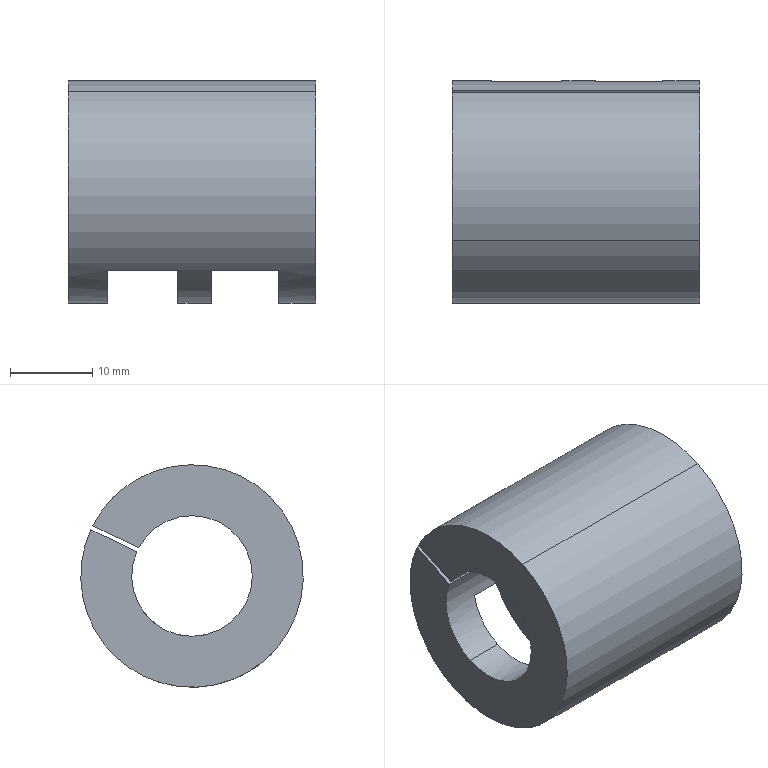Part | NX | 1 solid | 18 faces | box 30 x 27 x 27 mm | volume 9581 mm3 | plane 12 | cylinder 6 | commonest cylinder face diameters 14.64 x3 27 x3
STEP:
#1=CARTESIAN_POINT('',(15.301,-535.026,2413.504));
#2=VERTEX_POINT('',#1);
#3=CARTESIAN_POINT('',(15.301,-544.682,2416.678));
#4=VERTEX_POINT('',#3);
#5=CARTESIAN_POINT('',(15.301,-541.499,2410.086));
#6=DIRECTION('',(1.,0.,0.));
#7=DIRECTION('',(0.,-0.4348,0.9005));
#8=AXIS2_PLACEMENT_3D('',#5,#6,#7);
#9=CIRCLE('',#8,7.32);
#10=EDGE_CURVE('',#2,#4,#9,.T.);
#11=ORIENTED_EDGE('',*,*,#10,.T.);
#12=CARTESIAN_POINT('',(-14.699,-544.682,2416.678));
#13=VERTEX_POINT('',#12);
#14=CARTESIAN_POINT('',(15.301,-544.682,2416.678));
#15=DIRECTION('',(-1.,0.,0.));
#16=VECTOR('',#15,1.);
#17=LINE('',#14,#16);
#18=EDGE_CURVE('',#4,#13,#17,.T.);
#19=ORIENTED_EDGE('',*,*,#18,.T.);
#20=CARTESIAN_POINT('',(-14.699,-535.026,2413.504));
#21=VERTEX_POINT('',#20);
#22=CARTESIAN_POINT('',(-14.699,-541.499,2410.086));
#23=DIRECTION('',(1.,0.,0.));
#24=DIRECTION('',(0.,-0.4348,0.9005));
#25=AXIS2_PLACEMENT_3D('',#22,#23,#24);
#26=CIRCLE('',#25,7.32);
#27=EDGE_CURVE('',#21,#13,#26,.T.);
#28=ORIENTED_EDGE('',*,*,#27,.F.);
#29=CARTESIAN_POINT('',(15.301,-535.026,2413.504));
#30=DIRECTION('',(-1.,0.,0.));
#31=VECTOR('',#30,1.);
#32=LINE('',#29,#31);
#33=EDGE_CURVE('',#2,#21,#32,.T.);
#34=ORIENTED_EDGE('',*,*,#33,.F.);
#35=EDGE_LOOP('',(#11,#19,#28,#34));
#36=FACE_OUTER_BOUND('',#35,.T.);
#37=CARTESIAN_POINT('',(15.301,-541.499,2410.086));
#38=DIRECTION('',(-1.,0.,0.));
#39=DIRECTION('',(0.,0.4348,-0.9005));
#40=AXIS2_PLACEMENT_3D('',#37,#38,#39);
#41=CYLINDRICAL_SURFACE('',#40,7.32);
#42=ADVANCED_FACE('',(#36),#41,.F.);
#43=ORIENTED_EDGE('',*,*,#18,.F.);
#44=CARTESIAN_POINT('',(15.301,-538.317,2403.494));
#45=VERTEX_POINT('',#44);
#46=CARTESIAN_POINT('',(15.301,-541.499,2410.086));
#47=DIRECTION('',(1.,0.,0.));
#48=DIRECTION('',(0.,-0.4348,0.9005));
#49=AXIS2_PLACEMENT_3D('',#46,#47,#48);
#50=CIRCLE('',#49,7.32);
#51=EDGE_CURVE('',#4,#45,#50,.T.);
#52=ORIENTED_EDGE('',*,*,#51,.T.);
#53=CARTESIAN_POINT('',(10.819,-538.317,2403.494));
#54=VERTEX_POINT('',#53);
#55=CARTESIAN_POINT('',(15.301,-538.317,2403.494));
#56=DIRECTION('',(-1.,0.,0.));
#57=VECTOR('',#56,1.);
#58=LINE('',#55,#57);
#59=EDGE_CURVE('',#45,#54,#58,.T.);
#60=ORIENTED_EDGE('',*,*,#59,.T.);
#61=CARTESIAN_POINT('',(10.819,-544.91,2403.609));
#62=VERTEX_POINT('',#61);
#63=CARTESIAN_POINT('',(10.819,-541.499,2410.086));
#64=DIRECTION('',(1.,0.,0.));
#65=DIRECTION('',(0.,-0.4348,0.9005));
#66=AXIS2_PLACEMENT_3D('',#63,#64,#65);
#67=CIRCLE('',#66,7.32);
#68=EDGE_CURVE('',#62,#54,#67,.T.);
#69=ORIENTED_EDGE('',*,*,#68,.F.);
#70=CARTESIAN_POINT('',(2.647,-544.91,2403.609));
#71=VERTEX_POINT('',#70);
#72=CARTESIAN_POINT('',(15.301,-544.91,2403.609));
#73=DIRECTION('',(1.,0.,0.));
#74=VECTOR('',#73,1.);
#75=LINE('',#72,#74);
#76=EDGE_CURVE('',#71,#62,#75,.T.);
#77=ORIENTED_EDGE('',*,*,#76,.F.);
#78=CARTESIAN_POINT('',(2.647,-538.317,2403.494));
#79=VERTEX_POINT('',#78);
#80=CARTESIAN_POINT('',(2.647,-541.499,2410.086));
#81=DIRECTION('',(-1.,0.,0.));
#82=DIRECTION('',(0.,0.4348,-0.9005));
#83=AXIS2_PLACEMENT_3D('',#80,#81,#82);
#84=CIRCLE('',#83,7.32);
#85=EDGE_CURVE('',#79,#71,#84,.T.);
#86=ORIENTED_EDGE('',*,*,#85,.F.);
#87=CARTESIAN_POINT('',(-1.413,-538.317,2403.494));
#88=VERTEX_POINT('',#87);
#89=CARTESIAN_POINT('',(15.301,-538.317,2403.494));
#90=DIRECTION('',(-1.,0.,0.));
#91=VECTOR('',#90,1.);
#92=LINE('',#89,#91);
#93=EDGE_CURVE('',#79,#88,#92,.T.);
#94=ORIENTED_EDGE('',*,*,#93,.T.);
#95=CARTESIAN_POINT('',(-1.413,-544.91,2403.609));
#96=VERTEX_POINT('',#95);
#97=CARTESIAN_POINT('',(-1.413,-541.499,2410.086));
#98=DIRECTION('',(1.,0.,0.));
#99=DIRECTION('',(0.,-0.4348,0.9005));
#100=AXIS2_PLACEMENT_3D('',#97,#98,#99);
#101=CIRCLE('',#100,7.32);
#102=EDGE_CURVE('',#96,#88,#101,.T.);
#103=ORIENTED_EDGE('',*,*,#102,.F.);
#104=CARTESIAN_POINT('',(-9.954,-544.91,2403.609));
#105=VERTEX_POINT('',#104);
#106=CARTESIAN_POINT('',(15.301,-544.91,2403.609));
#107=DIRECTION('',(1.,0.,0.));
#108=VECTOR('',#107,1.);
#109=LINE('',#106,#108);
#110=EDGE_CURVE('',#105,#96,#109,.T.);
#111=ORIENTED_EDGE('',*,*,#110,.F.);
#112=CARTESIAN_POINT('',(-9.954,-538.317,2403.494));
#113=VERTEX_POINT('',#112);
#114=CARTESIAN_POINT('',(-9.954,-541.499,2410.086));
#115=DIRECTION('',(-1.,0.,0.));
#116=DIRECTION('',(0.,0.4348,-0.9005));
#117=AXIS2_PLACEMENT_3D('',#114,#115,#116);
#118=CIRCLE('',#117,7.32);
#119=EDGE_CURVE('',#113,#105,#118,.T.);
#120=ORIENTED_EDGE('',*,*,#119,.F.);
#121=CARTESIAN_POINT('',(-14.699,-538.317,2403.494));
#122=VERTEX_POINT('',#121);
#123=CARTESIAN_POINT('',(15.301,-538.317,2403.494));
#124=DIRECTION('',(-1.,0.,0.));
#125=VECTOR('',#124,1.);
#126=LINE('',#123,#125);
#127=EDGE_CURVE('',#113,#122,#126,.T.);
#128=ORIENTED_EDGE('',*,*,#127,.T.);
#129=CARTESIAN_POINT('',(-14.699,-541.499,2410.086));
#130=DIRECTION('',(1.,0.,0.));
#131=DIRECTION('',(0.,-0.4348,0.9005));
#132=AXIS2_PLACEMENT_3D('',#129,#130,#131);
#133=CIRCLE('',#132,7.32);
#134=EDGE_CURVE('',#13,#122,#133,.T.);
#135=ORIENTED_EDGE('',*,*,#134,.F.);
#136=EDGE_LOOP('',(#43,#52,#60,#69,#77,#86,#94,#103,#111,#120,#128,#135));
#137=FACE_OUTER_BOUND('',#136,.T.);
#138=CARTESIAN_POINT('',(15.301,-541.499,2410.086));
#139=DIRECTION('',(-1.,0.,0.));
#140=DIRECTION('',(0.,0.4348,-0.9005));
#141=AXIS2_PLACEMENT_3D('',#138,#139,#140);
#142=CYLINDRICAL_SURFACE('',#141,7.32);
#143=ADVANCED_FACE('',(#137),#142,.F.);
#144=CARTESIAN_POINT('',(15.301,-547.369,2422.243));
#145=VERTEX_POINT('',#144);
#146=CARTESIAN_POINT('',(15.301,-535.63,2397.929));
#147=VERTEX_POINT('',#146);
#148=CARTESIAN_POINT('',(15.301,-541.499,2410.086));
#149=DIRECTION('',(1.,0.,0.));
#150=DIRECTION('',(0.,-0.4348,0.9005));
#151=AXIS2_PLACEMENT_3D('',#148,#149,#150);
#152=CIRCLE('',#151,13.5);
#153=EDGE_CURVE('',#145,#147,#152,.T.);
#154=ORIENTED_EDGE('',*,*,#153,.F.);
#155=CARTESIAN_POINT('',(-14.699,-547.369,2422.243));
#156=VERTEX_POINT('',#155);
#157=CARTESIAN_POINT('',(15.301,-547.369,2422.243));
#158=DIRECTION('',(-1.,0.,0.));
#159=VECTOR('',#158,1.);
#160=LINE('',#157,#159);
#161=EDGE_CURVE('',#145,#156,#160,.T.);
#162=ORIENTED_EDGE('',*,*,#161,.T.);
#163=CARTESIAN_POINT('',(-14.699,-535.63,2397.929));
#164=VERTEX_POINT('',#163);
#165=CARTESIAN_POINT('',(-14.699,-541.499,2410.086));
#166=DIRECTION('',(1.,0.,0.));
#167=DIRECTION('',(0.,-0.4348,0.9005));
#168=AXIS2_PLACEMENT_3D('',#165,#166,#167);
#169=CIRCLE('',#168,13.5);
#170=EDGE_CURVE('',#156,#164,#169,.T.);
#171=ORIENTED_EDGE('',*,*,#170,.T.);
#172=CARTESIAN_POINT('',(-9.954,-535.63,2397.929));
#173=VERTEX_POINT('',#172);
#174=CARTESIAN_POINT('',(15.301,-535.63,2397.929));
#175=DIRECTION('',(-1.,0.,0.));
#176=VECTOR('',#175,1.);
#177=LINE('',#174,#176);
#178=EDGE_CURVE('',#173,#164,#177,.T.);
#179=ORIENTED_EDGE('',*,*,#178,.F.);
#180=CARTESIAN_POINT('',(-9.954,-551.117,2400.613));
#181=VERTEX_POINT('',#180);
#182=CARTESIAN_POINT('',(-9.954,-541.499,2410.086));
#183=DIRECTION('',(-1.,0.,0.));
#184=DIRECTION('',(0.,0.4348,-0.9005));
#185=AXIS2_PLACEMENT_3D('',#182,#183,#184);
#186=CIRCLE('',#185,13.5);
#187=EDGE_CURVE('',#173,#181,#186,.T.);
#188=ORIENTED_EDGE('',*,*,#187,.T.);
#189=CARTESIAN_POINT('',(-1.413,-551.117,2400.613));
#190=VERTEX_POINT('',#189);
#191=CARTESIAN_POINT('',(15.301,-551.117,2400.613));
#192=DIRECTION('',(1.,0.,0.));
#193=VECTOR('',#192,1.);
#194=LINE('',#191,#193);
#195=EDGE_CURVE('',#181,#190,#194,.T.);
#196=ORIENTED_EDGE('',*,*,#195,.T.);
#197=CARTESIAN_POINT('',(-1.413,-535.63,2397.929));
#198=VERTEX_POINT('',#197);
#199=CARTESIAN_POINT('',(-1.413,-541.499,2410.086));
#200=DIRECTION('',(1.,0.,0.));
#201=DIRECTION('',(0.,-0.4348,0.9005));
#202=AXIS2_PLACEMENT_3D('',#199,#200,#201);
#203=CIRCLE('',#202,13.5);
#204=EDGE_CURVE('',#190,#198,#203,.T.);
#205=ORIENTED_EDGE('',*,*,#204,.T.);
#206=CARTESIAN_POINT('',(2.647,-535.63,2397.929));
#207=VERTEX_POINT('',#206);
#208=CARTESIAN_POINT('',(15.301,-535.63,2397.929));
#209=DIRECTION('',(-1.,0.,0.));
#210=VECTOR('',#209,1.);
#211=LINE('',#208,#210);
#212=EDGE_CURVE('',#207,#198,#211,.T.);
#213=ORIENTED_EDGE('',*,*,#212,.F.);
#214=CARTESIAN_POINT('',(2.647,-551.117,2400.613));
#215=VERTEX_POINT('',#214);
#216=CARTESIAN_POINT('',(2.647,-541.499,2410.086));
#217=DIRECTION('',(-1.,0.,0.));
#218=DIRECTION('',(0.,0.4348,-0.9005));
#219=AXIS2_PLACEMENT_3D('',#216,#217,#218);
#220=CIRCLE('',#219,13.5);
#221=EDGE_CURVE('',#207,#215,#220,.T.);
#222=ORIENTED_EDGE('',*,*,#221,.T.);
#223=CARTESIAN_POINT('',(10.819,-551.117,2400.613));
#224=VERTEX_POINT('',#223);
#225=CARTESIAN_POINT('',(15.301,-551.117,2400.613));
#226=DIRECTION('',(1.,0.,0.));
#227=VECTOR('',#226,1.);
#228=LINE('',#225,#227);
#229=EDGE_CURVE('',#215,#224,#228,.T.);
#230=ORIENTED_EDGE('',*,*,#229,.T.);
#231=CARTESIAN_POINT('',(10.819,-535.63,2397.929));
#232=VERTEX_POINT('',#231);
#233=CARTESIAN_POINT('',(10.819,-541.499,2410.086));
#234=DIRECTION('',(1.,0.,0.));
#235=DIRECTION('',(0.,-0.4348,0.9005));
#236=AXIS2_PLACEMENT_3D('',#233,#234,#235);
#237=CIRCLE('',#236,13.5);
#238=EDGE_CURVE('',#224,#232,#237,.T.);
#239=ORIENTED_EDGE('',*,*,#238,.T.);
#240=CARTESIAN_POINT('',(15.301,-535.63,2397.929));
#241=DIRECTION('',(-1.,0.,0.));
#242=VECTOR('',#241,1.);
#243=LINE('',#240,#242);
#244=EDGE_CURVE('',#147,#232,#243,.T.);
#245=ORIENTED_EDGE('',*,*,#244,.F.);
#246=EDGE_LOOP('',(#154,#162,#171,#179,#188,#196,#205,#213,#222,#230,#239,#245));
#247=FACE_OUTER_BOUND('',#246,.T.);
#248=CARTESIAN_POINT('',(15.301,-541.499,2410.086));
#249=DIRECTION('',(-1.,0.,0.));
#250=DIRECTION('',(0.,0.4348,-0.9005));
#251=AXIS2_PLACEMENT_3D('',#248,#249,#250);
#252=CYLINDRICAL_SURFACE('',#251,13.5);
#253=ADVANCED_FACE('',(#247),#252,.T.);
#254=CARTESIAN_POINT('',(15.301,-529.23,2415.717));
#255=VERTEX_POINT('',#254);
#256=CARTESIAN_POINT('',(15.301,-541.499,2410.086));
#257=DIRECTION('',(1.,0.,0.));
#258=DIRECTION('',(0.,-0.4348,0.9005));
#259=AXIS2_PLACEMENT_3D('',#256,#257,#258);
#260=CIRCLE('',#259,13.5);
#261=EDGE_CURVE('',#147,#255,#260,.T.);
#262=ORIENTED_EDGE('',*,*,#261,.F.);
#263=ORIENTED_EDGE('',*,*,#244,.T.);
#264=CARTESIAN_POINT('',(10.819,-528.099,2411.726));
#265=VERTEX_POINT('',#264);
#266=CARTESIAN_POINT('',(10.819,-541.499,2410.086));
#267=DIRECTION('',(1.,0.,0.));
#268=DIRECTION('',(0.,-0.4348,0.9005));
#269=AXIS2_PLACEMENT_3D('',#266,#267,#268);
#270=CIRCLE('',#269,13.5);
#271=EDGE_CURVE('',#232,#265,#270,.T.);
#272=ORIENTED_EDGE('',*,*,#271,.T.);
#273=CARTESIAN_POINT('',(2.647,-528.099,2411.726));
#274=VERTEX_POINT('',#273);
#275=CARTESIAN_POINT('',(15.301,-528.099,2411.726));
#276=DIRECTION('',(-1.,0.,0.));
#277=VECTOR('',#276,1.);
#278=LINE('',#275,#277);
#279=EDGE_CURVE('',#265,#274,#278,.T.);
#280=ORIENTED_EDGE('',*,*,#279,.T.);
#281=CARTESIAN_POINT('',(2.647,-541.499,2410.086));
#282=DIRECTION('',(-1.,0.,0.));
#283=DIRECTION('',(0.,0.4348,-0.9005));
#284=AXIS2_PLACEMENT_3D('',#281,#282,#283);
#285=CIRCLE('',#284,13.5);
#286=EDGE_CURVE('',#274,#207,#285,.T.);
#287=ORIENTED_EDGE('',*,*,#286,.T.);
#288=ORIENTED_EDGE('',*,*,#212,.T.);
#289=CARTESIAN_POINT('',(-1.413,-528.099,2411.726));
#290=VERTEX_POINT('',#289);
#291=CARTESIAN_POINT('',(-1.413,-541.499,2410.086));
#292=DIRECTION('',(1.,0.,0.));
#293=DIRECTION('',(0.,-0.4348,0.9005));
#294=AXIS2_PLACEMENT_3D('',#291,#292,#293);
#295=CIRCLE('',#294,13.5);
#296=EDGE_CURVE('',#198,#290,#295,.T.);
#297=ORIENTED_EDGE('',*,*,#296,.T.);
#298=CARTESIAN_POINT('',(-9.954,-528.099,2411.726));
#299=VERTEX_POINT('',#298);
#300=CARTESIAN_POINT('',(15.301,-528.099,2411.726));
#301=DIRECTION('',(-1.,0.,0.));
#302=VECTOR('',#301,1.);
#303=LINE('',#300,#302);
#304=EDGE_CURVE('',#290,#299,#303,.T.);
#305=ORIENTED_EDGE('',*,*,#304,.T.);
#306=CARTESIAN_POINT('',(-9.954,-541.499,2410.086));
#307=DIRECTION('',(-1.,0.,0.));
#308=DIRECTION('',(0.,0.4348,-0.9005));
#309=AXIS2_PLACEMENT_3D('',#306,#307,#308);
#310=CIRCLE('',#309,13.5);
#311=EDGE_CURVE('',#299,#173,#310,.T.);
#312=ORIENTED_EDGE('',*,*,#311,.T.);
#313=ORIENTED_EDGE('',*,*,#178,.T.);
#314=CARTESIAN_POINT('',(-14.699,-529.23,2415.717));
#315=VERTEX_POINT('',#314);
#316=CARTESIAN_POINT('',(-14.699,-541.499,2410.086));
#317=DIRECTION('',(1.,0.,0.));
#318=DIRECTION('',(0.,-0.4348,0.9005));
#319=AXIS2_PLACEMENT_3D('',#316,#317,#318);
#320=CIRCLE('',#319,13.5);
#321=EDGE_CURVE('',#164,#315,#320,.T.);
#322=ORIENTED_EDGE('',*,*,#321,.T.);
#323=CARTESIAN_POINT('',(15.301,-529.23,2415.717));
#324=DIRECTION('',(1.,0.,0.));
#325=VECTOR('',#324,1.);
#326=LINE('',#323,#325);
#327=EDGE_CURVE('',#315,#255,#326,.T.);
#328=ORIENTED_EDGE('',*,*,#327,.T.);
#329=EDGE_LOOP('',(#262,#263,#272,#280,#287,#288,#297,#305,#312,#313,#322,#328));
#330=FACE_OUTER_BOUND('',#329,.T.);
#331=CARTESIAN_POINT('',(15.301,-541.499,2410.086));
#332=DIRECTION('',(-1.,0.,0.));
#333=DIRECTION('',(0.,0.4348,-0.9005));
#334=AXIS2_PLACEMENT_3D('',#331,#332,#333);
#335=CYLINDRICAL_SURFACE('',#334,13.5);
#336=ADVANCED_FACE('',(#330),#335,.T.);
#337=CARTESIAN_POINT('',(15.301,-534.797,2413.029));
#338=VERTEX_POINT('',#337);
#339=CARTESIAN_POINT('',(15.301,-528.162,2416.233));
#340=DIRECTION('',(0.,0.9005,0.4348));
#341=VECTOR('',#340,1.);
#342=LINE('',#339,#341);
#343=EDGE_CURVE('',#338,#255,#342,.T.);
#344=ORIENTED_EDGE('',*,*,#343,.F.);
#345=CARTESIAN_POINT('',(15.301,-541.499,2410.086));
#346=DIRECTION('',(1.,0.,0.));
#347=DIRECTION('',(0.,-0.4348,0.9005));
#348=AXIS2_PLACEMENT_3D('',#345,#346,#347);
#349=CIRCLE('',#348,7.32);
#350=EDGE_CURVE('',#45,#338,#349,.T.);
#351=ORIENTED_EDGE('',*,*,#350,.F.);
#352=ORIENTED_EDGE('',*,*,#51,.F.);
#353=ORIENTED_EDGE('',*,*,#10,.F.);
#354=CARTESIAN_POINT('',(15.301,-529.459,2416.192));
#355=VERTEX_POINT('',#354);
#356=CARTESIAN_POINT('',(15.301,-528.391,2416.708));
#357=DIRECTION('',(0.,-0.9005,-0.4348));
#358=VECTOR('',#357,1.);
#359=LINE('',#356,#358);
#360=EDGE_CURVE('',#355,#2,#359,.T.);
#361=ORIENTED_EDGE('',*,*,#360,.F.);
#362=CARTESIAN_POINT('',(15.301,-541.499,2410.086));
#363=DIRECTION('',(1.,0.,0.));
#364=DIRECTION('',(0.,-0.4348,0.9005));
#365=AXIS2_PLACEMENT_3D('',#362,#363,#364);
#366=CIRCLE('',#365,13.5);
#367=EDGE_CURVE('',#355,#145,#366,.T.);
#368=ORIENTED_EDGE('',*,*,#367,.T.);
#369=ORIENTED_EDGE('',*,*,#153,.T.);
#370=ORIENTED_EDGE('',*,*,#261,.T.);
#371=EDGE_LOOP('',(#344,#351,#352,#353,#361,#368,#369,#370));
#372=FACE_OUTER_BOUND('',#371,.T.);
#373=CARTESIAN_POINT('',(15.301,-541.499,2410.086));
#374=DIRECTION('',(1.,0.,0.));
#375=DIRECTION('',(0.,-0.4348,0.9005));
#376=AXIS2_PLACEMENT_3D('',#373,#374,#375);
#377=PLANE('',#376);
#378=ADVANCED_FACE('',(#372),#377,.T.);
#379=ORIENTED_EDGE('',*,*,#27,.T.);
#380=ORIENTED_EDGE('',*,*,#134,.T.);
#381=CARTESIAN_POINT('',(-14.699,-534.797,2413.029));
#382=VERTEX_POINT('',#381);
#383=CARTESIAN_POINT('',(-14.699,-541.499,2410.086));
#384=DIRECTION('',(1.,0.,0.));
#385=DIRECTION('',(0.,-0.4348,0.9005));
#386=AXIS2_PLACEMENT_3D('',#383,#384,#385);
#387=CIRCLE('',#386,7.32);
#388=EDGE_CURVE('',#122,#382,#387,.T.);
#389=ORIENTED_EDGE('',*,*,#388,.T.);
#390=CARTESIAN_POINT('',(-14.699,-528.162,2416.233));
#391=DIRECTION('',(0.,0.9005,0.4348));
#392=VECTOR('',#391,1.);
#393=LINE('',#390,#392);
#394=EDGE_CURVE('',#382,#315,#393,.T.);
#395=ORIENTED_EDGE('',*,*,#394,.T.);
#396=ORIENTED_EDGE('',*,*,#321,.F.);
#397=ORIENTED_EDGE('',*,*,#170,.F.);
#398=CARTESIAN_POINT('',(-14.699,-529.459,2416.192));
#399=VERTEX_POINT('',#398);
#400=CARTESIAN_POINT('',(-14.699,-541.499,2410.086));
#401=DIRECTION('',(1.,0.,0.));
#402=DIRECTION('',(0.,-0.4348,0.9005));
#403=AXIS2_PLACEMENT_3D('',#400,#401,#402);
#404=CIRCLE('',#403,13.5);
#405=EDGE_CURVE('',#399,#156,#404,.T.);
#406=ORIENTED_EDGE('',*,*,#405,.F.);
#407=CARTESIAN_POINT('',(-14.699,-528.391,2416.708));
#408=DIRECTION('',(0.,-0.9005,-0.4348));
#409=VECTOR('',#408,1.);
#410=LINE('',#407,#409);
#411=EDGE_CURVE('',#399,#21,#410,.T.);
#412=ORIENTED_EDGE('',*,*,#411,.T.);
#413=EDGE_LOOP('',(#379,#380,#389,#395,#396,#397,#406,#412));
#414=FACE_OUTER_BOUND('',#413,.T.);
#415=CARTESIAN_POINT('',(-14.699,-541.499,2410.086));
#416=DIRECTION('',(1.,0.,0.));
#417=DIRECTION('',(0.,-0.4348,0.9005));
#418=AXIS2_PLACEMENT_3D('',#415,#416,#417);
#419=PLANE('',#418);
#420=ADVANCED_FACE('',(#414),#419,.F.);
#421=ORIENTED_EDGE('',*,*,#161,.F.);
#422=ORIENTED_EDGE('',*,*,#367,.F.);
#423=CARTESIAN_POINT('',(15.301,-529.459,2416.192));
#424=DIRECTION('',(-1.,0.,0.));
#425=VECTOR('',#424,1.);
#426=LINE('',#423,#425);
#427=EDGE_CURVE('',#355,#399,#426,.T.);
#428=ORIENTED_EDGE('',*,*,#427,.T.);
#429=ORIENTED_EDGE('',*,*,#405,.T.);
#430=EDGE_LOOP('',(#421,#422,#428,#429));
#431=FACE_OUTER_BOUND('',#430,.T.);
#432=CARTESIAN_POINT('',(15.301,-541.499,2410.086));
#433=DIRECTION('',(-1.,0.,0.));
#434=DIRECTION('',(0.,0.4348,-0.9005));
#435=AXIS2_PLACEMENT_3D('',#432,#433,#434);
#436=CYLINDRICAL_SURFACE('',#435,13.5);
#437=ADVANCED_FACE('',(#431),#436,.T.);
#438=ORIENTED_EDGE('',*,*,#59,.F.);
#439=ORIENTED_EDGE('',*,*,#350,.T.);
#440=CARTESIAN_POINT('',(15.301,-534.797,2413.029));
#441=DIRECTION('',(1.,0.,0.));
#442=VECTOR('',#441,1.);
#443=LINE('',#440,#442);
#444=EDGE_CURVE('',#382,#338,#443,.T.);
#445=ORIENTED_EDGE('',*,*,#444,.F.);
#446=ORIENTED_EDGE('',*,*,#388,.F.);
#447=ORIENTED_EDGE('',*,*,#127,.F.);
#448=CARTESIAN_POINT('',(-9.954,-534.306,2408.729));
#449=VERTEX_POINT('',#448);
#450=CARTESIAN_POINT('',(-9.954,-541.499,2410.086));
#451=DIRECTION('',(-1.,0.,0.));
#452=DIRECTION('',(0.,0.4348,-0.9005));
#453=AXIS2_PLACEMENT_3D('',#450,#451,#452);
#454=CIRCLE('',#453,7.32);
#455=EDGE_CURVE('',#449,#113,#454,.T.);
#456=ORIENTED_EDGE('',*,*,#455,.F.);
#457=CARTESIAN_POINT('',(-1.413,-534.306,2408.729));
#458=VERTEX_POINT('',#457);
#459=CARTESIAN_POINT('',(15.301,-534.306,2408.729));
#460=DIRECTION('',(-1.,0.,0.));
#461=VECTOR('',#460,1.);
#462=LINE('',#459,#461);
#463=EDGE_CURVE('',#458,#449,#462,.T.);
#464=ORIENTED_EDGE('',*,*,#463,.F.);
#465=CARTESIAN_POINT('',(-1.413,-541.499,2410.086));
#466=DIRECTION('',(1.,0.,0.));
#467=DIRECTION('',(0.,-0.4348,0.9005));
#468=AXIS2_PLACEMENT_3D('',#465,#466,#467);
#469=CIRCLE('',#468,7.32);
#470=EDGE_CURVE('',#88,#458,#469,.T.);
#471=ORIENTED_EDGE('',*,*,#470,.F.);
#472=ORIENTED_EDGE('',*,*,#93,.F.);
#473=CARTESIAN_POINT('',(2.647,-534.306,2408.729));
#474=VERTEX_POINT('',#473);
#475=CARTESIAN_POINT('',(2.647,-541.499,2410.086));
#476=DIRECTION('',(-1.,0.,0.));
#477=DIRECTION('',(0.,0.4348,-0.9005));
#478=AXIS2_PLACEMENT_3D('',#475,#476,#477);
#479=CIRCLE('',#478,7.32);
#480=EDGE_CURVE('',#474,#79,#479,.T.);
#481=ORIENTED_EDGE('',*,*,#480,.F.);
#482=CARTESIAN_POINT('',(10.819,-534.306,2408.729));
#483=VERTEX_POINT('',#482);
#484=CARTESIAN_POINT('',(15.301,-534.306,2408.729));
#485=DIRECTION('',(-1.,0.,0.));
#486=VECTOR('',#485,1.);
#487=LINE('',#484,#486);
#488=EDGE_CURVE('',#483,#474,#487,.T.);
#489=ORIENTED_EDGE('',*,*,#488,.F.);
#490=CARTESIAN_POINT('',(10.819,-541.499,2410.086));
#491=DIRECTION('',(1.,0.,0.));
#492=DIRECTION('',(0.,-0.4348,0.9005));
#493=AXIS2_PLACEMENT_3D('',#490,#491,#492);
#494=CIRCLE('',#493,7.32);
#495=EDGE_CURVE('',#54,#483,#494,.T.);
#496=ORIENTED_EDGE('',*,*,#495,.F.);
#497=EDGE_LOOP('',(#438,#439,#445,#446,#447,#456,#464,#471,#472,#481,#489,#496));
#498=FACE_OUTER_BOUND('',#497,.T.);
#499=CARTESIAN_POINT('',(15.301,-541.499,2410.086));
#500=DIRECTION('',(-1.,0.,0.));
#501=DIRECTION('',(0.,0.4348,-0.9005));
#502=AXIS2_PLACEMENT_3D('',#499,#500,#501);
#503=CYLINDRICAL_SURFACE('',#502,7.32);
#504=ADVANCED_FACE('',(#498),#503,.F.);
#505=ORIENTED_EDGE('',*,*,#360,.T.);
#506=ORIENTED_EDGE('',*,*,#33,.T.);
#507=ORIENTED_EDGE('',*,*,#411,.F.);
#508=ORIENTED_EDGE('',*,*,#427,.F.);
#509=EDGE_LOOP('',(#505,#506,#507,#508));
#510=FACE_OUTER_BOUND('',#509,.T.);
#511=CARTESIAN_POINT('',(-14.699,-528.391,2416.708));
#512=DIRECTION('',(0.,-0.4348,0.9005));
#513=DIRECTION('',(0.,-0.9005,-0.4348));
#514=AXIS2_PLACEMENT_3D('',#511,#512,#513);
#515=PLANE('',#514);
#516=ADVANCED_FACE('',(#510),#515,.F.);
#517=ORIENTED_EDGE('',*,*,#394,.F.);
#518=ORIENTED_EDGE('',*,*,#444,.T.);
#519=ORIENTED_EDGE('',*,*,#343,.T.);
#520=ORIENTED_EDGE('',*,*,#327,.F.);
#521=EDGE_LOOP('',(#517,#518,#519,#520));
#522=FACE_OUTER_BOUND('',#521,.T.);
#523=CARTESIAN_POINT('',(-14.699,-528.162,2416.233));
#524=DIRECTION('',(0.,0.4348,-0.9005));
#525=DIRECTION('',(1.,0.,0.));
#526=AXIS2_PLACEMENT_3D('',#523,#524,#525);
#527=PLANE('',#526);
#528=ADVANCED_FACE('',(#522),#527,.F.);
#529=CARTESIAN_POINT('',(-9.954,-527.453,2412.038));
#530=DIRECTION('',(0.,-0.9005,-0.4348));
#531=VECTOR('',#530,1.);
#532=LINE('',#529,#531);
#533=EDGE_CURVE('',#299,#449,#532,.T.);
#534=ORIENTED_EDGE('',*,*,#533,.T.);
#535=ORIENTED_EDGE('',*,*,#455,.T.);
#536=ORIENTED_EDGE('',*,*,#119,.T.);
#537=CARTESIAN_POINT('',(-9.954,-527.453,2412.038));
#538=DIRECTION('',(0.,-0.9005,-0.4348));
#539=VECTOR('',#538,1.);
#540=LINE('',#537,#539);
#541=EDGE_CURVE('',#105,#181,#540,.T.);
#542=ORIENTED_EDGE('',*,*,#541,.T.);
#543=ORIENTED_EDGE('',*,*,#187,.F.);
#544=ORIENTED_EDGE('',*,*,#311,.F.);
#545=EDGE_LOOP('',(#534,#535,#536,#542,#543,#544));
#546=FACE_OUTER_BOUND('',#545,.T.);
#547=CARTESIAN_POINT('',(-9.954,-523.144,2403.111));
#548=DIRECTION('',(-1.,0.,0.));
#549=DIRECTION('',(0.,0.4348,-0.9005));
#550=AXIS2_PLACEMENT_3D('',#547,#548,#549);
#551=PLANE('',#550);
#552=ADVANCED_FACE('',(#546),#551,.F.);
#553=CARTESIAN_POINT('',(-1.413,-527.453,2412.038));
#554=DIRECTION('',(0.,-0.9005,-0.4348));
#555=VECTOR('',#554,1.);
#556=LINE('',#553,#555);
#557=EDGE_CURVE('',#290,#458,#556,.T.);
#558=ORIENTED_EDGE('',*,*,#557,.T.);
#559=ORIENTED_EDGE('',*,*,#463,.T.);
#560=ORIENTED_EDGE('',*,*,#533,.F.);
#561=ORIENTED_EDGE('',*,*,#304,.F.);
#562=EDGE_LOOP('',(#558,#559,#560,#561));
#563=FACE_OUTER_BOUND('',#562,.T.);
#564=CARTESIAN_POINT('',(-9.954,-527.453,2412.038));
#565=DIRECTION('',(0.,-0.4348,0.9005));
#566=DIRECTION('',(-1.,0.,0.));
#567=AXIS2_PLACEMENT_3D('',#564,#565,#566);
#568=PLANE('',#567);
#569=ADVANCED_FACE('',(#563),#568,.F.);
#570=ORIENTED_EDGE('',*,*,#541,.F.);
#571=ORIENTED_EDGE('',*,*,#110,.T.);
#572=CARTESIAN_POINT('',(-1.413,-527.453,2412.038));
#573=DIRECTION('',(0.,-0.9005,-0.4348));
#574=VECTOR('',#573,1.);
#575=LINE('',#572,#574);
#576=EDGE_CURVE('',#96,#190,#575,.T.);
#577=ORIENTED_EDGE('',*,*,#576,.T.);
#578=ORIENTED_EDGE('',*,*,#195,.F.);
#579=EDGE_LOOP('',(#570,#571,#577,#578));
#580=FACE_OUTER_BOUND('',#579,.T.);
#581=CARTESIAN_POINT('',(-9.954,-527.453,2412.038));
#582=DIRECTION('',(0.,-0.4348,0.9005));
#583=DIRECTION('',(-1.,0.,0.));
#584=AXIS2_PLACEMENT_3D('',#581,#582,#583);
#585=PLANE('',#584);
#586=ADVANCED_FACE('',(#580),#585,.F.);
#587=ORIENTED_EDGE('',*,*,#576,.F.);
#588=ORIENTED_EDGE('',*,*,#102,.T.);
#589=ORIENTED_EDGE('',*,*,#470,.T.);
#590=ORIENTED_EDGE('',*,*,#557,.F.);
#591=ORIENTED_EDGE('',*,*,#296,.F.);
#592=ORIENTED_EDGE('',*,*,#204,.F.);
#593=EDGE_LOOP('',(#587,#588,#589,#590,#591,#592));
#594=FACE_OUTER_BOUND('',#593,.T.);
#595=CARTESIAN_POINT('',(-1.413,-523.144,2403.111));
#596=DIRECTION('',(1.,0.,0.));
#597=DIRECTION('',(0.,-0.4348,0.9005));
#598=AXIS2_PLACEMENT_3D('',#595,#596,#597);
#599=PLANE('',#598);
#600=ADVANCED_FACE('',(#594),#599,.F.);
#601=CARTESIAN_POINT('',(2.647,-527.453,2412.038));
#602=DIRECTION('',(0.,-0.9005,-0.4348));
#603=VECTOR('',#602,1.);
#604=LINE('',#601,#603);
#605=EDGE_CURVE('',#274,#474,#604,.T.);
#606=ORIENTED_EDGE('',*,*,#605,.T.);
#607=ORIENTED_EDGE('',*,*,#480,.T.);
#608=ORIENTED_EDGE('',*,*,#85,.T.);
#609=CARTESIAN_POINT('',(2.647,-527.453,2412.038));
#610=DIRECTION('',(0.,-0.9005,-0.4348));
#611=VECTOR('',#610,1.);
#612=LINE('',#609,#611);
#613=EDGE_CURVE('',#71,#215,#612,.T.);
#614=ORIENTED_EDGE('',*,*,#613,.T.);
#615=ORIENTED_EDGE('',*,*,#221,.F.);
#616=ORIENTED_EDGE('',*,*,#286,.F.);
#617=EDGE_LOOP('',(#606,#607,#608,#614,#615,#616));
#618=FACE_OUTER_BOUND('',#617,.T.);
#619=CARTESIAN_POINT('',(2.647,-523.144,2403.111));
#620=DIRECTION('',(-1.,0.,0.));
#621=DIRECTION('',(0.,0.4348,-0.9005));
#622=AXIS2_PLACEMENT_3D('',#619,#620,#621);
#623=PLANE('',#622);
#624=ADVANCED_FACE('',(#618),#623,.F.);
#625=CARTESIAN_POINT('',(10.819,-527.453,2412.038));
#626=DIRECTION('',(0.,-0.9005,-0.4348));
#627=VECTOR('',#626,1.);
#628=LINE('',#625,#627);
#629=EDGE_CURVE('',#265,#483,#628,.T.);
#630=ORIENTED_EDGE('',*,*,#629,.T.);
#631=ORIENTED_EDGE('',*,*,#488,.T.);
#632=ORIENTED_EDGE('',*,*,#605,.F.);
#633=ORIENTED_EDGE('',*,*,#279,.F.);
#634=EDGE_LOOP('',(#630,#631,#632,#633));
#635=FACE_OUTER_BOUND('',#634,.T.);
#636=CARTESIAN_POINT('',(2.647,-527.453,2412.038));
#637=DIRECTION('',(0.,-0.4348,0.9005));
#638=DIRECTION('',(-1.,0.,0.));
#639=AXIS2_PLACEMENT_3D('',#636,#637,#638);
#640=PLANE('',#639);
#641=ADVANCED_FACE('',(#635),#640,.F.);
#642=ORIENTED_EDGE('',*,*,#613,.F.);
#643=ORIENTED_EDGE('',*,*,#76,.T.);
#644=CARTESIAN_POINT('',(10.819,-527.453,2412.038));
#645=DIRECTION('',(0.,-0.9005,-0.4348));
#646=VECTOR('',#645,1.);
#647=LINE('',#644,#646);
#648=EDGE_CURVE('',#62,#224,#647,.T.);
#649=ORIENTED_EDGE('',*,*,#648,.T.);
#650=ORIENTED_EDGE('',*,*,#229,.F.);
#651=EDGE_LOOP('',(#642,#643,#649,#650));
#652=FACE_OUTER_BOUND('',#651,.T.);
#653=CARTESIAN_POINT('',(2.647,-527.453,2412.038));
#654=DIRECTION('',(0.,-0.4348,0.9005));
#655=DIRECTION('',(-1.,0.,0.));
#656=AXIS2_PLACEMENT_3D('',#653,#654,#655);
#657=PLANE('',#656);
#658=ADVANCED_FACE('',(#652),#657,.F.);
#659=ORIENTED_EDGE('',*,*,#648,.F.);
#660=ORIENTED_EDGE('',*,*,#68,.T.);
#661=ORIENTED_EDGE('',*,*,#495,.T.);
#662=ORIENTED_EDGE('',*,*,#629,.F.);
#663=ORIENTED_EDGE('',*,*,#271,.F.);
#664=ORIENTED_EDGE('',*,*,#238,.F.);
#665=EDGE_LOOP('',(#659,#660,#661,#662,#663,#664));
#666=FACE_OUTER_BOUND('',#665,.T.);
#667=CARTESIAN_POINT('',(10.819,-523.144,2403.111));
#668=DIRECTION('',(1.,0.,0.));
#669=DIRECTION('',(0.,-0.4348,0.9005));
#670=AXIS2_PLACEMENT_3D('',#667,#668,#669);
#671=PLANE('',#670);
#672=ADVANCED_FACE('',(#666),#671,.F.);
#673=CLOSED_SHELL('',(#42,#143,#253,#336,#378,#420,#437,#504,#516,#528,#552,#569,#586,#600,#624,#641,#658,#672));
#674=MANIFOLD_SOLID_BREP('',#673);
#675=(LENGTH_UNIT()NAMED_UNIT(*)SI_UNIT(.MILLI.,.METRE.));
#676=UNCERTAINTY_MEASURE_WITH_UNIT(LENGTH_MEASURE(0.00002),#675,'','');
#677=(NAMED_UNIT(*)PLANE_ANGLE_UNIT()SI_UNIT($,.RADIAN.));
#678=PLANE_ANGLE_MEASURE_WITH_UNIT(PLANE_ANGLE_MEASURE(0.01745),#677);
#679=DIMENSIONAL_EXPONENTS(0.,0.,0.,0.,0.,0.,0.);
#680=(CONVERSION_BASED_UNIT('DEGREE',#678)NAMED_UNIT(#679)PLANE_ANGLE_UNIT());
#681=(NAMED_UNIT(*)SI_UNIT($,.STERADIAN.)SOLID_ANGLE_UNIT());
#682=(GEOMETRIC_REPRESENTATION_CONTEXT(3)GLOBAL_UNCERTAINTY_ASSIGNED_CONTEXT((#676))GLOBAL_UNIT_ASSIGNED_CONTEXT((#675,#680,#681))REPRESENTATION_CONTEXT('',''));
#683=ADVANCED_BREP_SHAPE_REPRESENTATION('',(#674),#682);